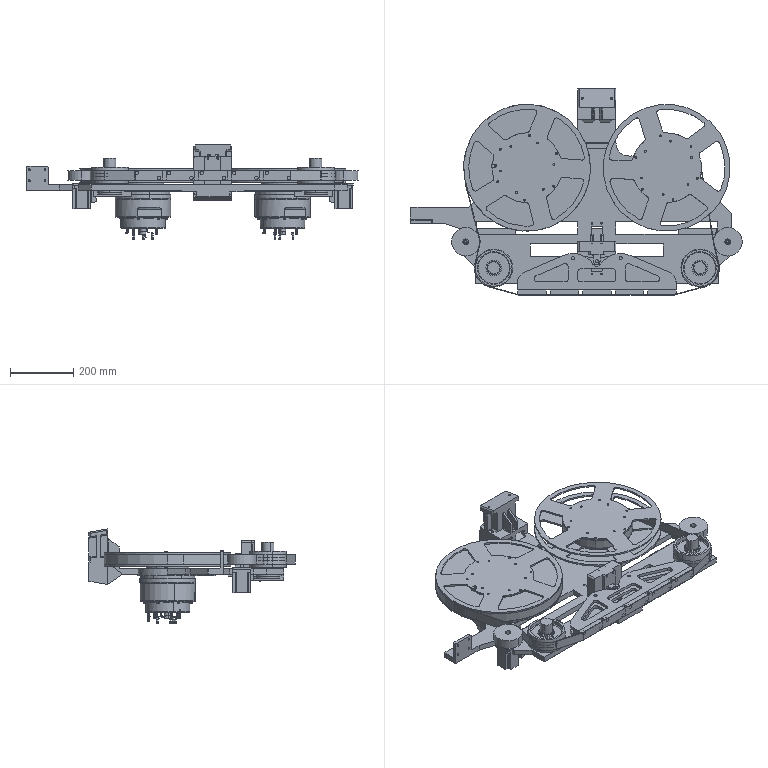Part | STEP file | 打磨单元方案20250311-1-第二版 | 180 solids | 6987 faces | volume 21551656 mm3 | plane 2600 | cylinder 2413 | cone 1396 | spline 372 | torus 126 | sphere 80 | commonest cylinder face diameters 6 x298 5 x240 6.6 x216 5.5 x160 10 x154 3 x146